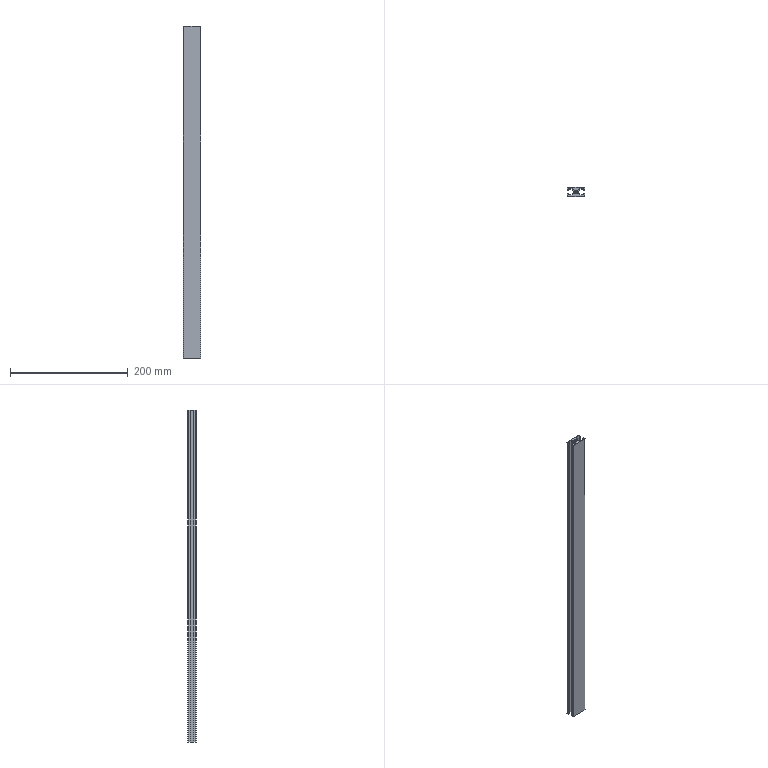Part | SolidWorks | features BaseBody 1, MoveFace 1 | 1 solid | 53 faces | box 30 x 15 x 565 mm | volume 136260 mm3 | plane 38 | cylinder 15 | commonest cylinder face diameters 1 x6 5 x5 2 x4